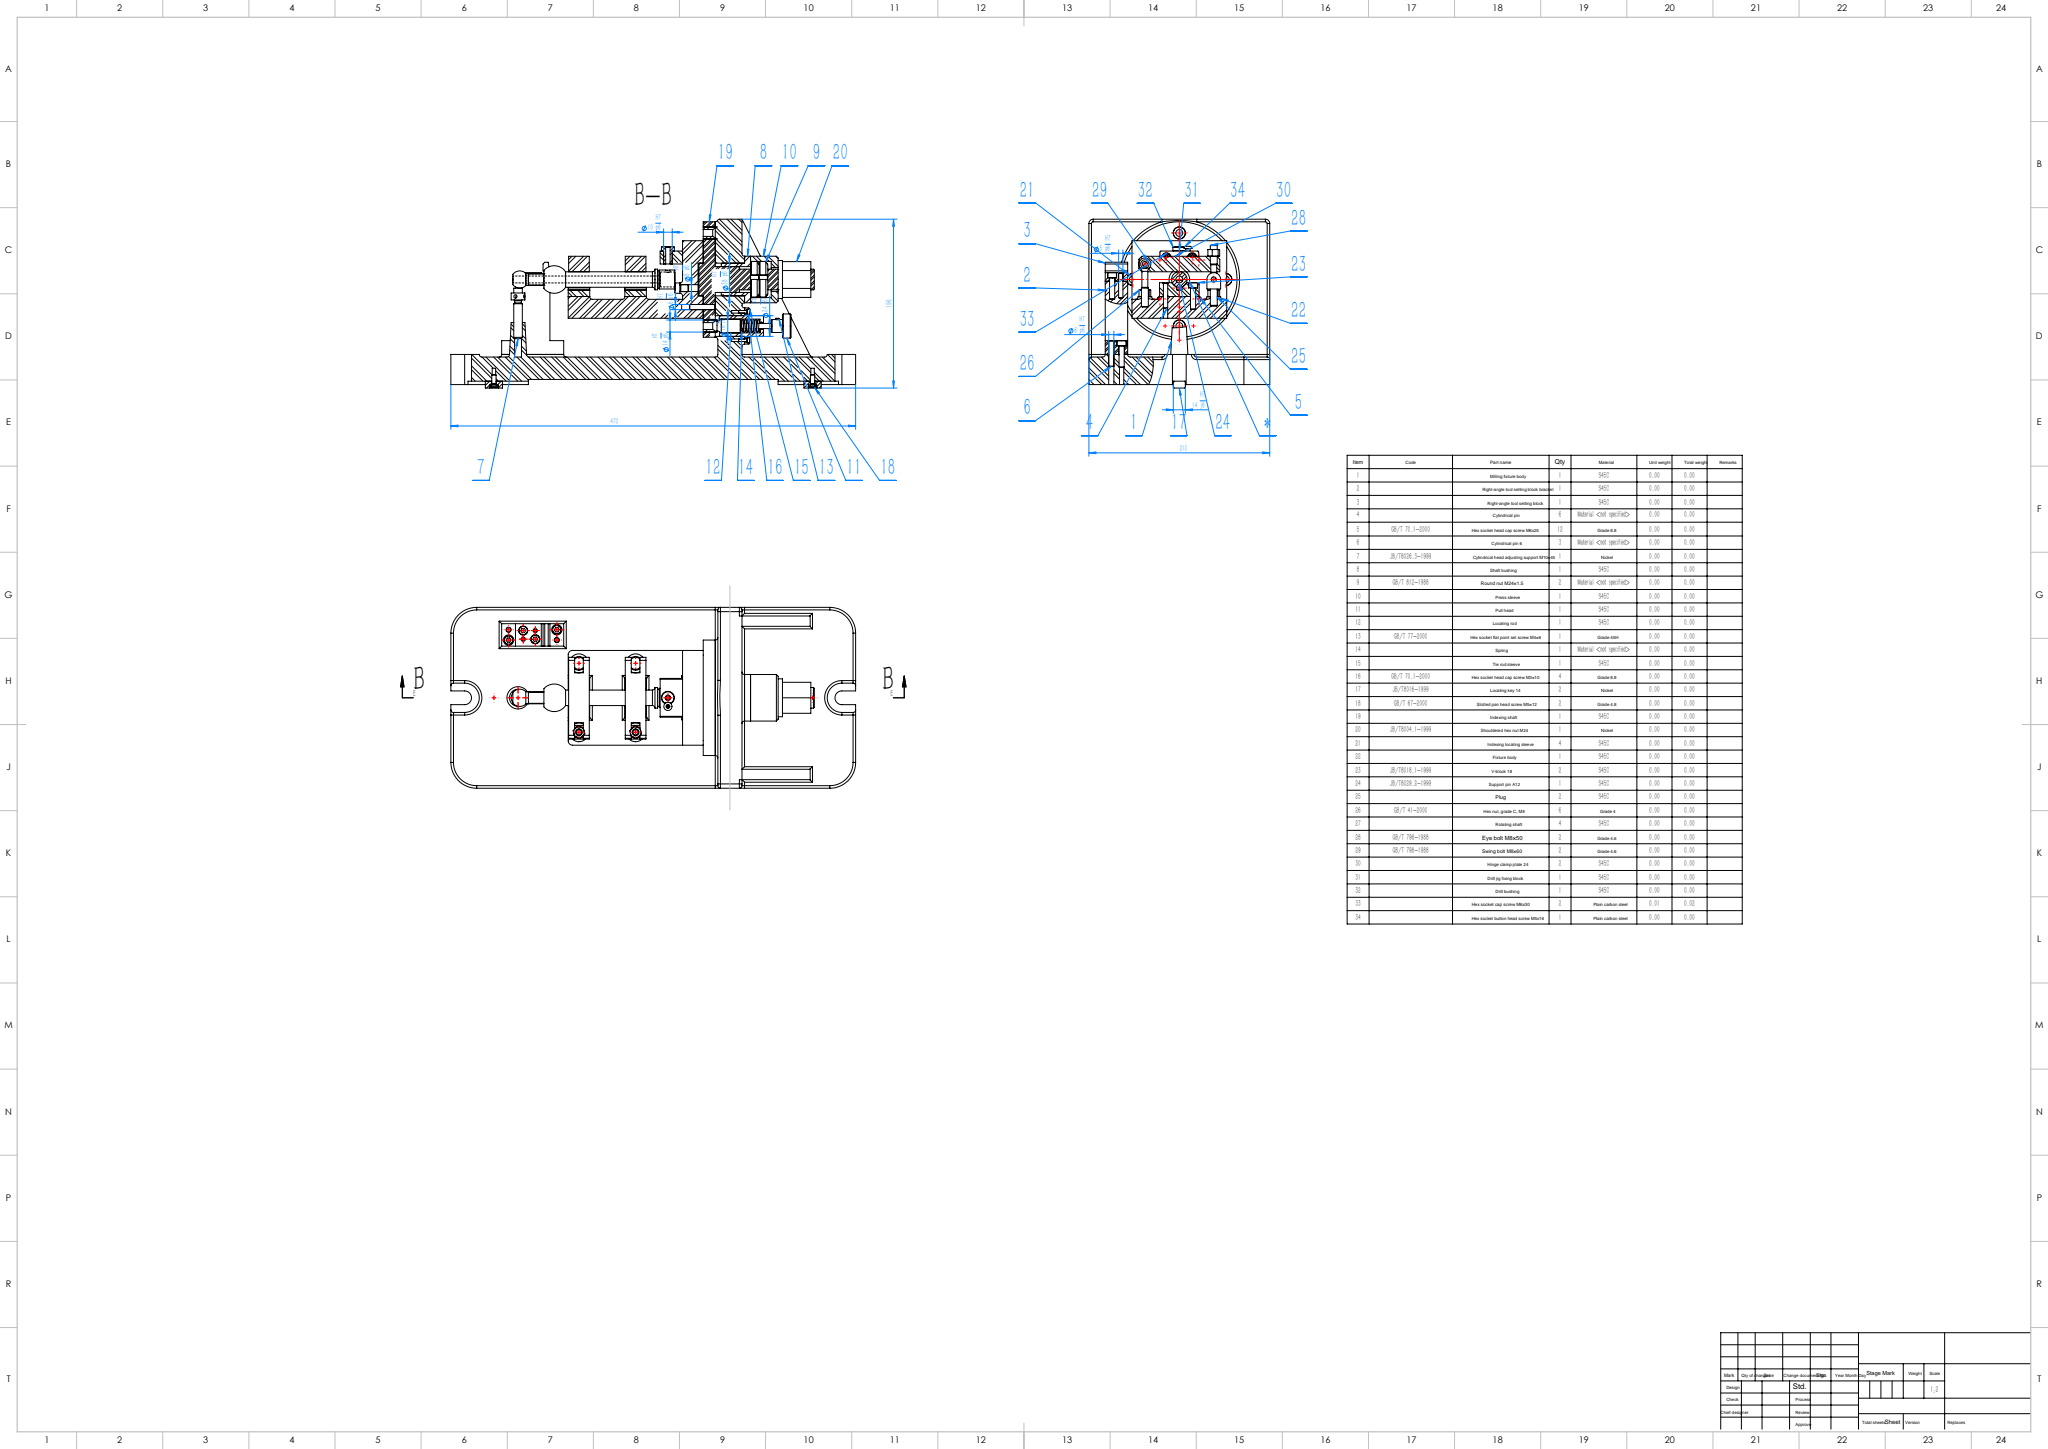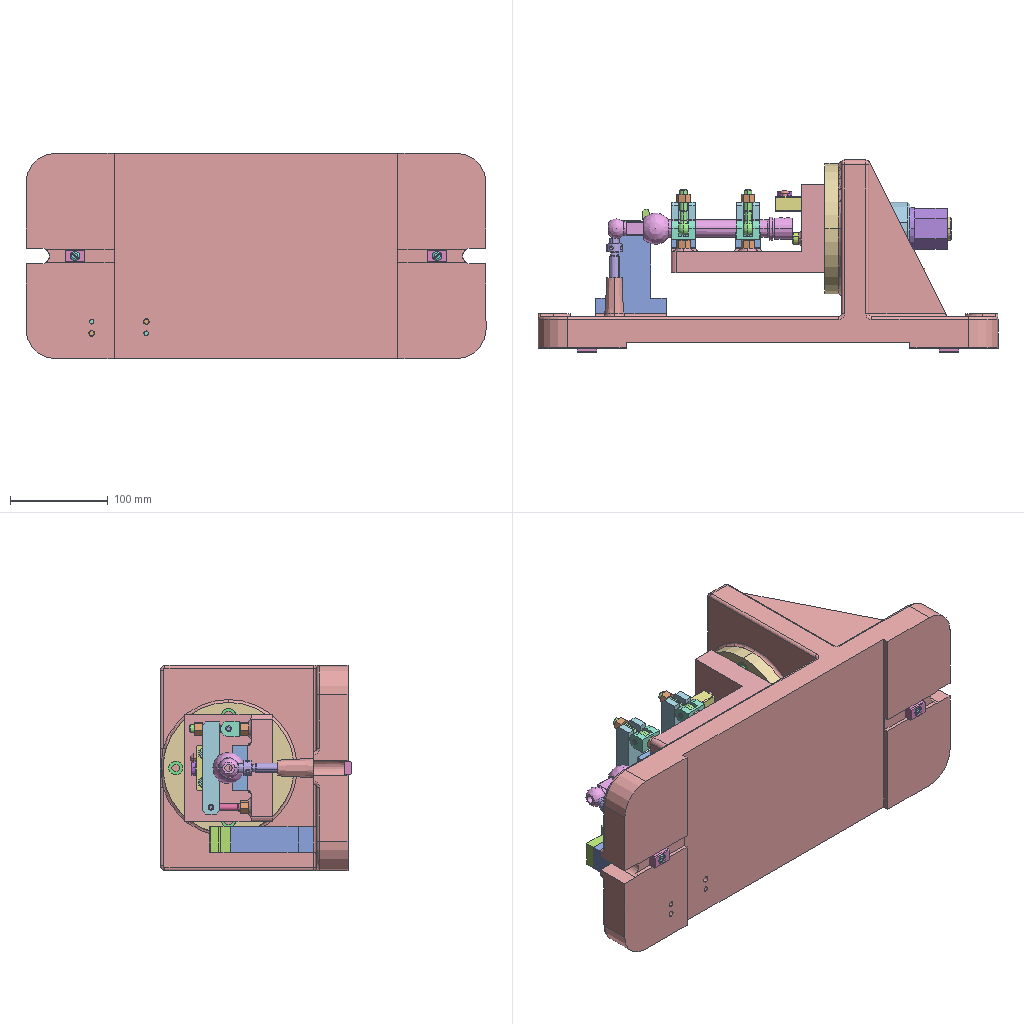Assembly | SolidWorks | 38 different items | 80 placed | box 470 x 196 x 210 mm
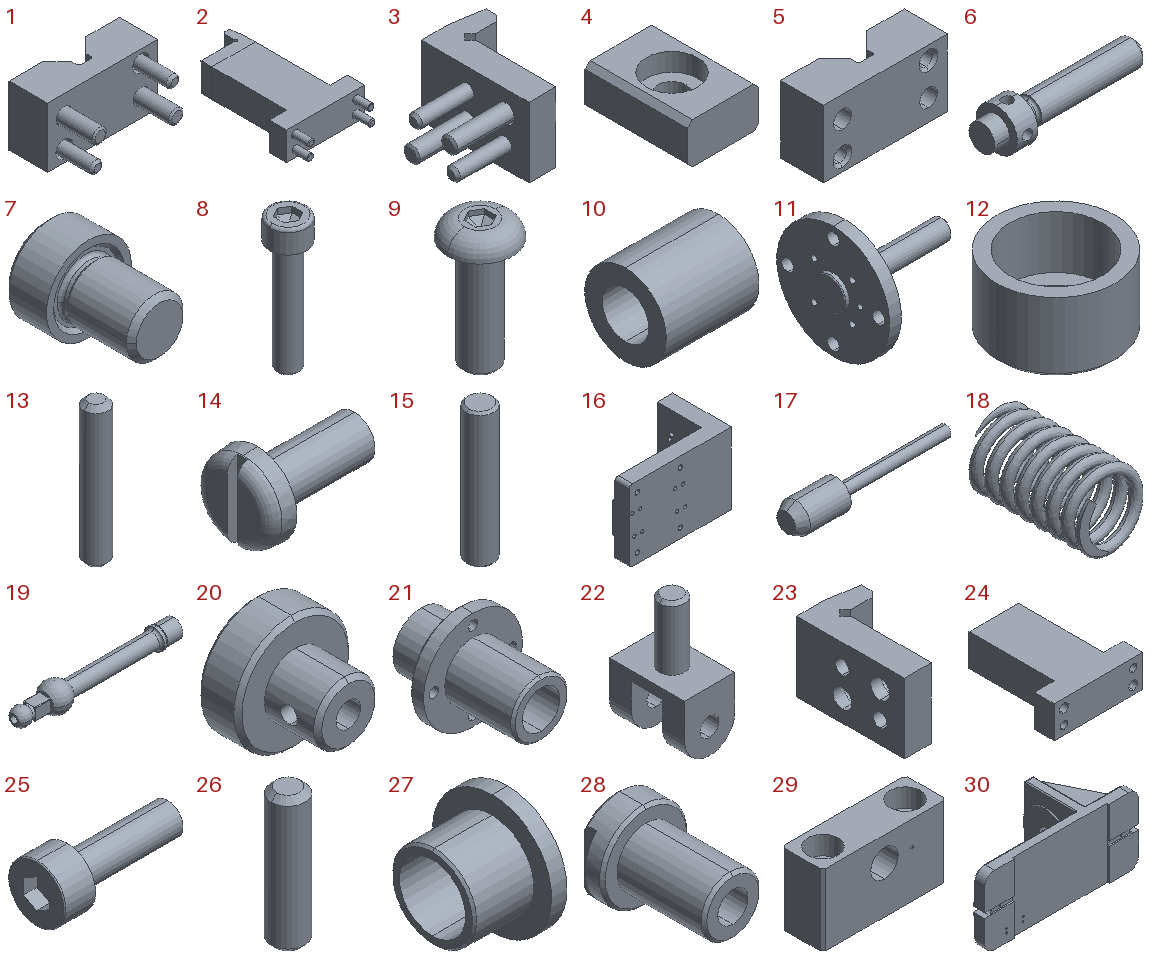Parts list (item | name | quantity | parent item | size | volume | features):
1 | (subassembly) | x2 | - | 46 x 31 x 25 mm | 16828 mm3 | features AEMSimFeature 1, CompositeCurve 1
2 | (subassembly) | x1 | - | 72 x 122.018 x 26 mm | 115436 mm3 | features CompositeCurve 2, AEMSimFeature 1
3 | (subassembly) | x1 | in 2 | 43 x 40 x 26 mm | 14025 mm3 | features CompositeCurve 1
4 | - | x2 | - | 14 x 20 x 8 mm | 1818 mm3 | features Cut 2, Chamfer 1, Extrusion 1
5 | - | x2 | in 1 | 46 x 16 x 25 mm | 13455 mm3 | features Chamfer 4, Cut 3, Fillet 2, Extrusion 1
6 | - | x1 | - | 58.66 x 16 x 16 mm | 5066 mm3 | features Boss 2, Cut 2, Chamfer 1, Extrusion 1, Fillet 1, ICE 1, Revolution 1
7 | - | x1 | - | 12 x 16 x 12 mm | 1142 mm3 | features Revolution 1
8 | - | x2 | - | 10 x 10 x 36 mm | 1267 mm3 | features Chamfer 2, Fillet 2, ICE 2, Extrusion 1, RefAxis 1
9 | - | x1 | - | 9.5 x 9.5 x 18.5 mm | 446.572 mm3 | features Chamfer 2, Fillet 2, ICE 2, Extrusion 1, RefAxis 1
10 | - | x4 | - | 16 x 14 x 14 mm | 1434 mm3 | features Revolution 1
11 | - | x1 | - | 134 x 134 x 134 mm | 249153 mm3 | features ICE 8, Chamfer 2, CirPattern 2, Revolution 1
12 | - | x1 | - | 54 x 54 x 32 mm | 34780 mm3 | features Chamfer 1, Extrusion 1, ICE 1
13 | - | x6 | in 1, 3 | 5 x 5 x 30 mm | 575.435 mm3 | features Chamfer 1, Extrusion 1
14 | - | x2 | - | 15 x 9.5 x 9.5 mm | 406.666 mm3 | features Cut 1, LPattern 1, RevCut 1, Revolution 1
15 | - | x3 | in 2 | 6 x 6 x 30 mm | 843.779 mm3 | features Chamfer 1, Extrusion 1
16 | - | x1 | - | 156.771 x 90 x 110 mm | 550567 mm3 | features ICE 7, Fillet 2, Cut 1, Extrusion 1, HoleWzd 1
17 | - | x1 | - | 86 x 16 x 16 mm | 6778 mm3 | features Revolution 1
18 | - | x1 | - | 13.98 x 23 x 13.98 mm | 890.57 mm3 | features Helix 1, ICE 1, RefAxis 1, Sweep 1
19 | - | x1 | - | 188 x 32 x 32 mm | 46322 mm3 | features ICE 2, Revolution 1
20 | - | x1 | - | 28 x 23 x 28 mm | 7638 mm3 | features ICE 2, Chamfer 1, Extrusion 1
21 | - | x1 | - | 42 x 51 x 42 mm | 18428 mm3 | features ICE 4, Chamfer 1, CirPattern 1, Extrusion 1
22 | - | x2 | - | 16 x 24 x 39 mm | 4949 mm3 | features ICE 3, Chamfer 1, Extrusion 1
23 | - | x1 | in 3 | 22.018 x 40 x 26 mm | 10653 mm3 | features ICE 2, Extrusion 1
24 | - | x1 | in 2 | 72 x 85 x 26 mm | 97502 mm3 | features ICE 4, Extrusion 1
25 | - | x4 | - | 13 x 5.5 x 5.5 mm | 134.591 mm3 | features BlendCut 1, Cut 1, Fillet 1, LPattern 1, RevCut 1, Revolution 1
26 | - | x4 | - | 6 x 6 x 24 mm | 661.829 mm3 | features Chamfer 1, Extrusion 1
27 | - | x1 | - | 34 x 54 x 54 mm | 22561 mm3 | features Chamfer 1, Revolution 1
28 | - | x1 | - | 15 x 20 x 15 mm | 1593 mm3 | features ICE 2, Chamfer 1, Extrusion 1
29 | - | x1 | - | 45 x 15 x 26 mm | 12916 mm3 | features HoleWzd 3, Chamfer 1, Cut 1, Extrusion 1
30 | - | x1 | - | 470 x 192 x 210 mm | 3845072 mm3 | features ICE 10, Fillet 4, Cut 2, Draft 1, Extrusion 1
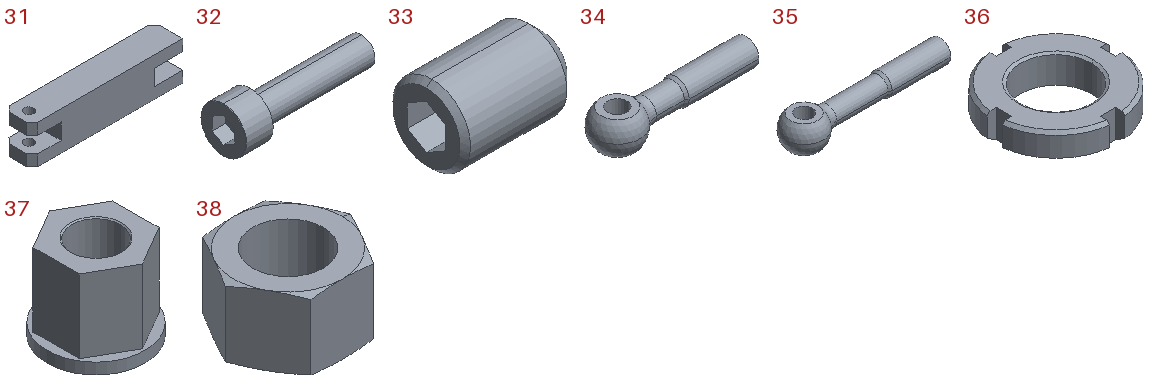31 | - | x2 | - | 94 x 18 x 24 mm | 33475 mm3 | features Chamfer 2, ICE 2, Extrusion 1
32 | - | x12 | in 1, 2, 3 | 31 x 10 x 10 mm | 1111 mm3 | features BlendCut 1, Cut 1, Fillet 1, LPattern 1, RevCut 1, Revolution 1
33 | - | x1 | - | 6 x 4 x 4 mm | 66.123 mm3 | features RevCut 2, Cut 1, LPattern 1, Revolution 1
34 | - | x2 | - | 47 x 14 x 10 mm | 2546 mm3 | features Cut 2, Revolution 2, Chamfer 1, Fillet 1, LPattern 1, RevCut 1
35 | - | x2 | - | 57 x 14 x 10 mm | 2922 mm3 | features Cut 2, Revolution 2, Chamfer 1, Fillet 1, LPattern 1, RevCut 1
36 | - | x2 | - | 41.664 x 41.664 x 10 mm | 8085 mm3 | features Chamfer 3, CirPattern 1, Cut 1, Extrusion 1
37 | - | x1 | - | 44 x 44 x 38 mm | 30187 mm3 | features 3DProfileFeature 1, Boss 1, Chamfer 1, Extrusion 1, HoleWzd 1, RevCut 1
38 | - | x6 | - | 14.2 x 12.298 x 7.9 mm | 635.641 mm3 | features Cut 2, Chamfer 1, Extrusion 1
Mates (type | each side: item.copy, entity, surface, feature):
In the top assembly
Coincident | 30.1 face plane Boss-Extrude2 | 24.1 face plane Boss-Extrude1
Coincident | 30.1 edge | 24.1 face plane Boss-Extrude1 | 2 times
Concentric | 30.1 face cylinder Boss-Extrude4 | 6.1 face cylinder Boss-Extrude
Concentric | 30.1 face cylinder Cut-Extrude4 | 27.1 face cylinder Revolve1
Coincident | 30.1 face plane Boss-Extrude6 | 27.1 face plane Revolve1
Concentric | 27.1 face cylinder Revolve1 | 36.1 face cylinder Boss-Extrude
Coincident | 27.1 face plane Revolve1 | 36.1 face plane Boss-Extrude
Concentric | 36.1 face cylinder Boss-Extrude | 36.2 face cylinder Boss-Extrude
Coincident | 36.1 face plane Boss-Extrude | 36.2 face plane Boss-Extrude
Concentric | 27.1 face cylinder Revolve1 | 12.1 face cylinder Boss-Extrude1
Coincident | 27.1 face plane Revolve1 | 12.1 edge
Concentric | 20.1 face cylinder Boss-Extrude1 | 17.1 face cylinder Revolve1
Coincident | 20.1 face plane Boss-Extrude1 | 17.1 edge
Concentric | 20.1 face cylinder Cut-Extrude1 | 33.1 face cylinder Boss-Revolve
Tangent | 17.1 face cylinder Revolve1 | 33.1 face plane Boss-Revolve
Concentric | 30.1 face cylinder Cut-Extrude4 | 17.1 face cylinder Revolve1
Coincident | 17.1 axis | 18.1 axis
Coincident | 17.1 face plane Revolve1 | 18.1 face plane Cut-Extrude1
Concentric | 30.1 face cylinder Cut-Extrude4 | 21.1 face cylinder Boss-Extrude1
Coincident | 30.1 face plane Boss-Extrude6 | 21.1 face plane Boss-Extrude2
Parallel | 30.1 face plane Boss-Extrude3 | 21.1 plane
DistanceDim | 21.1 face plane Boss-Extrude1 | 20.1 face plane Boss-Extrude1
Coincident | 21.1 face plane Boss-Extrude2 | 25.1 face plane Boss-Revolve
Concentric | 21.1 face cylinder CirPattern1 | 25.1 face cylinder Boss-Revolve
Coincident | 30.1 face plane Cut-Extrude3 | 4.1 face plane Boss-Extrude | 2 times
DistanceDim | 4.1 face plane Boss-Extrude | 30.1 face plane Boss-Extrude1
Coincident | 4.1 face plane Cut-Extrude1 | 14.1 face plane Boss-Revolve
Concentric | 4.1 face cylinder Cut-Extrude2 | 14.1 face cylinder Boss-Revolve
Concentric | 11.1 face cylinder Cut-Extrude4 | 15.1 face cylinder Boss-Extrude1
Coincident | 11.1 face plane Boss-Extrude1 | 15.1 face plane Boss-Extrude1
Coincident | 11.1 face plane Boss-Extrude1 | 32.1 face plane Boss-Revolve
Concentric | 11.1 face cylinder Cut-Extrude5 | 32.1 face cylinder Boss-Revolve
Concentric | 12.1 face cylinder Boss-Extrude1 | 11.1 face cylinder Revolve1
Concentric | 21.1 face cylinder Boss-Extrude1 | 11.1 face cylinder Cut-Extrude6
Coincident | 30.1 face plane Boss-Extrude5 | 11.1 face plane Boss-Extrude1
Concentric | 11.1 face cylinder Revolve1 | 37.1 face cylinder M24x2.0 Tapped Hole1
Coincident | 12.1 face plane Boss-Extrude1 | 37.1 face plane Boss-Extrude
Parallel | 30.1 face plane Boss-Extrude3 | 37.1 face plane Boss-Extrude1
Concentric | 11.1 face cylinder Cut-Extrude6 | 10.1 face cylinder Revolve1
Coincident | 11.1 face plane Boss-Extrude1 | 10.1 face plane Revolve1
Concentric | 11.1 face cylinder Boss-Extrude1 | 16.1 face cylinder Cut-Extrude3
Parallel | 30.1 face plane Boss-Extrude3 | 16.1 face plane Boss-Extrude1
Coincident | 11.1 face plane Boss-Extrude1 | 16.1 face plane Boss-Extrude1
Coincident | 16.1 face plane Boss-Extrude4 | 5.1 face plane Boss-Extrude
Coincident | 16.1 edge | 5.1 face plane Boss-Extrude | 2 times
Coincident | 16.1 edge | 7.1 face cylinder Boss-Revolve
Coincident | 16.1 face plane Boss-Extrude5 | 7.1 face plane Boss-Revolve
Tangent | 5.1 face plane Cut-Extrude1 | 19.1 face cylinder Revolve1 | 2 times
Coincident | 7.1 face plane Boss-Revolve | 19.1 face plane Revolve1
Tangent | 6.1 face plane Cut-Extrude3 | 19.1 face sphere Revolve1
Parallel | 16.1 face plane Boss-Extrude1 | 19.1 face plane Cut-Extrude1
Concentric | 16.1 edge | 38.1 face cylinder Boss-Extrude
Coincident | 16.1 face plane Boss-Extrude3 | 38.1 face plane Boss-Extrude
Concentric | 22.1 face cylinder Boss-Extrude2 | 38.1 face cylinder Boss-Extrude
Parallel | 16.1 face plane Boss-Extrude1 | 22.1 face plane Boss-Extrude1
Coincident | 22.1 edge | 26.1 face cylinder Boss-Extrude1
Coincident | 22.1 face plane Boss-Extrude1 | 26.1 face plane Boss-Extrude1
Concentric | 26.1 face cylinder Boss-Extrude1 | 34.1 face cylinder Cut-Extrude2
Coincident | 22.1 face plane Cut-Extrude1 | 34.1 face plane Cut-Extrude1
Parallel | 16.1 face plane Boss-Extrude1 | 34.1 face plane Boss-Revolve1
Concentric | 16.1 face cylinder Boss-Extrude1 | 35.1 face cylinder Boss-Revolve1
Parallel | 16.1 face plane Boss-Extrude1 | 35.1 face plane Cut-Extrude1
Coincident | 22.1 face plane Boss-Extrude1 | 26.2 face plane Boss-Extrude1
Concentric | 35.1 face cylinder Cut-Extrude2 | 26.2 face cylinder Boss-Extrude1
Concentric | 26.2 face cylinder Boss-Extrude1 | 31.1 face cylinder Cut-Extrude2
Parallel | 16.1 face plane Boss-Extrude2 | 31.1 face plane Boss-Extrude1
Tangent | 19.1 face cylinder Revolve1 | 31.1 face plane Boss-Extrude1
Coincident | 35.1 face plane Cut-Extrude1 | 31.1 face plane Cut-Extrude1
DistanceDim | 22.1 face plane Boss-Extrude1 | 16.1 face plane Boss-Extrude1
Concentric | 34.1 face cylinder Boss-Revolve1 | 38.2 face cylinder Boss-Extrude
Coincident | 31.1 face plane Boss-Extrude1 | 38.2 face plane Boss-Extrude
Concentric | 35.1 face cylinder Boss-Revolve1 | 38.3 face cylinder Boss-Extrude
Coincident | 16.1 face plane Boss-Extrude3 | 38.3 face plane Boss-Extrude
Coincident | 16.1 face plane Boss-Extrude2 | 29.1 face plane Boss-Extrude1
Width | 16.1 face plane Boss-Extrude1 | 16.1 face plane Boss-Extrude1 | 29.1 face plane Boss-Extrude1 | 29.1 face plane Boss-Extrude1
DistanceDim | 29.1 face plane Boss-Extrude1 | 16.1 face plane Boss-Extrude2
Concentric | 29.1 face cylinder Cut-Extrude1 | 28.1 face cylinder Boss-Extrude1
Coincident | 29.1 face plane Boss-Extrude1 | 28.1 face plane Boss-Extrude2
Coincident | 29.1 face plane CBORE for M6 Hexagon socket head cap screws1 | 8.1 plane
Concentric | 16.1 face cylinder M6 Tapped Hole1 | 8.1 axis
Coincident | 29.1 face plane CBORE for M6 Hexagon socket head cap screws1 | 8.2 plane
Concentric | 16.1 face cylinder M6 Tapped Hole1 | 8.2 axis
Parallel | 16.1 face plane Boss-Extrude1 | 28.1 face plane Cut-Extrude1
Coincident | 28.1 face plane Cut-Extrude1 | 9.1 plane
Concentric | 29.1 face cylinder M5 Tapped Hole1 | 9.1 axis
Parallel | 30.1 face plane Boss-Extrude3 | 20.1 plane
Parallel | 30.1 face plane Boss-Extrude1 | 11.1 plane
In subassembly 1
Coincident | 5.2 face plane Boss-Extrude | 13.1 face plane Boss-Extrude1
Coincident | 5.2 face plane Cut-Extrude5 | 32.1 edge
Concentric | 5.2 face cylinder Cut-Extrude4 | 32.1 face cylinder Boss-Revolve
Coincident | 32.1 face plane Boss-Revolve | 32.2 face plane Boss-Revolve
Concentric | 5.2 face cylinder Cut-Extrude4 | 32.2 face cylinder Boss-Revolve
In subassembly 2
Coincident | 24.2 face plane Boss-Extrude1 | 23.1 face plane Boss-Extrude1
Coincident | 24.2 face plane Boss-Extrude2 | 23.1 face plane Boss-Extrude1 | 2 times
Concentric | 24.2 face cylinder Cut-Extrude1 | 15.1 face cylinder Boss-Extrude1
Coincident | 24.2 face plane Boss-Extrude1 | 15.1 face plane Boss-Extrude1
Coincident | 24.2 face plane Boss-Extrude1 | 15.2 face plane Boss-Extrude1
Concentric | 24.2 face cylinder Cut-Extrude1 | 15.2 face cylinder Boss-Extrude1
Coincident | 24.2 face plane Cut-Extrude2 | 32.1 edge
Concentric | 24.2 face cylinder Cut-Extrude2 | 32.1 face cylinder Boss-Revolve
Concentric | 24.2 face cylinder Cut-Extrude2 | 32.2 face cylinder Boss-Revolve
Coincident | 24.2 face plane Cut-Extrude2 | 32.2 edge
In subassembly 3
Concentric | 23.2 face cylinder Cut-Extrude2 | 32.1 face cylinder Boss-Revolve
Coincident | 23.2 face plane Cut-Extrude2 | 32.1 edge
Concentric | 23.2 face cylinder Cut-Extrude2 | 32.2 face cylinder Boss-Revolve
Coincident | 32.1 face plane Boss-Revolve | 32.2 face plane Boss-Revolve
Coincident | 23.2 face plane Boss-Extrude1 | 13.1 face plane Boss-Extrude1
Concentric | 23.2 face cylinder Cut-Extrude1 | 13.1 face cylinder Boss-Extrude1
Coincident | 23.2 face plane Boss-Extrude1 | 13.2 face plane Boss-Extrude1
Concentric | 23.2 face cylinder Cut-Extrude1 | 13.2 face cylinder Boss-Extrude1